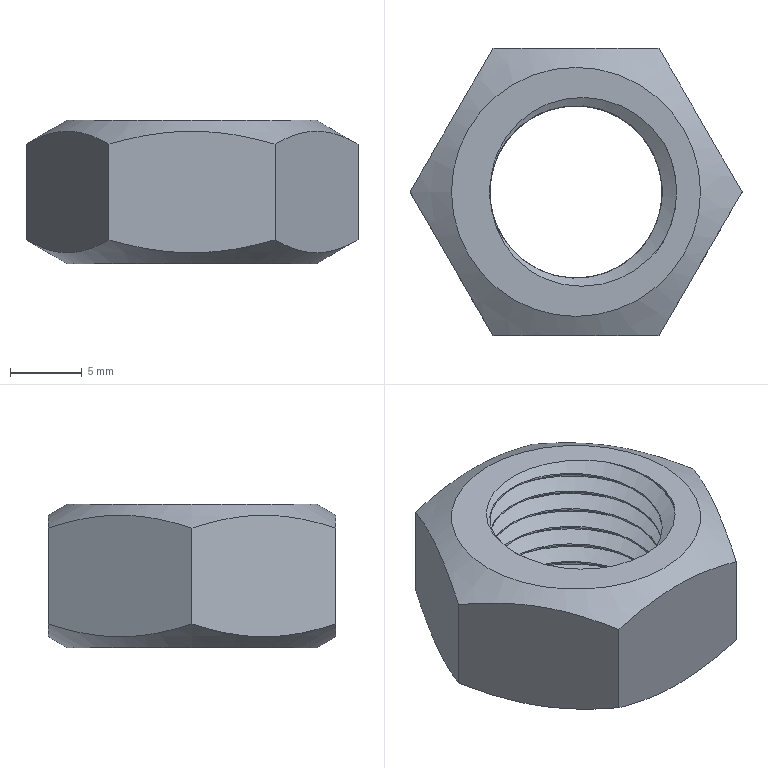Part | NX | features DATUM_CSYS 3, SKETCH 2, EXTRUDE 1, SWP104 1, THREADS 1 | 1 solid | 14 faces | box 23.094 x 20 x 10 mm | volume 1985 mm3 | plane 8 | cylinder 2 | spline 2 | cone 2 | commonest cylinder face diameters 12 x1 14 x1